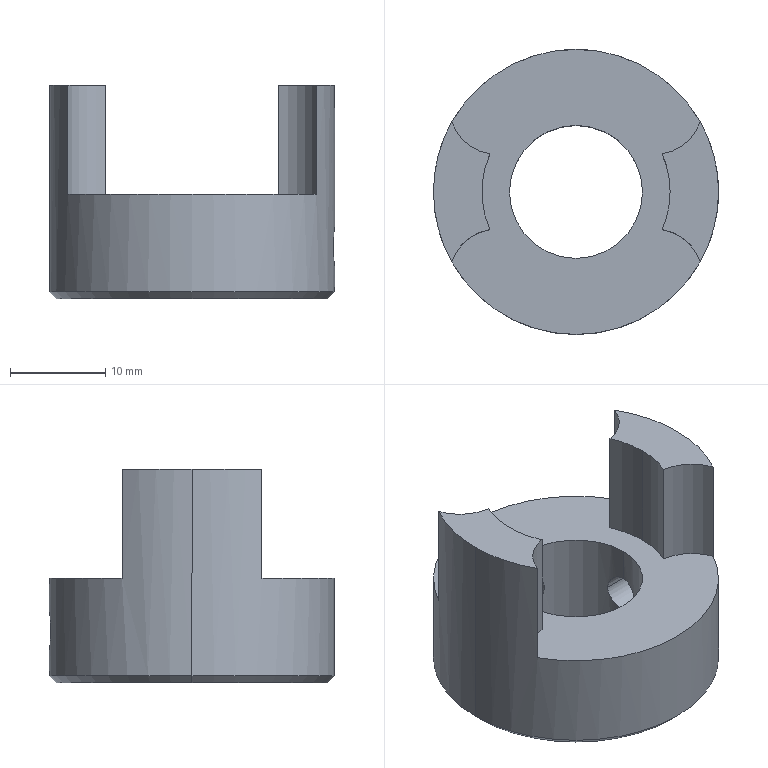Part | SolidWorks | features BaseBody 1 | 1 solid | 21 faces | box 30 x 30 x 22.5 mm | volume 7120 mm3 | cylinder 15 | plane 4 | cone 2 | commonest cylinder face diameters 4 x4 10 x4 19.8 x3 14 x2 30 x2
STEP:
#1=CARTESIAN_POINT('',(0.,15.,-14.));
#2=VERTEX_POINT('',#1);
#3=CARTESIAN_POINT('',(0.,15.,-10.));
#4=VERTEX_POINT('',#3);
#5=CARTESIAN_POINT('',(0.,15.,-14.));
#6=CARTESIAN_POINT('',(0.1323,15.,-14.));
#7=CARTESIAN_POINT('',(0.2623,14.998,-13.987));
#8=CARTESIAN_POINT('',(0.5181,14.992,-13.936));
#9=CARTESIAN_POINT('',(0.6452,14.987,-13.898));
#10=CARTESIAN_POINT('',(0.8873,14.974,-13.797));
#11=CARTESIAN_POINT('',(1.002,14.967,-13.736));
#12=CARTESIAN_POINT('',(1.219,14.951,-13.591));
#13=CARTESIAN_POINT('',(1.322,14.942,-13.506));
#14=CARTESIAN_POINT('',(1.599,14.916,-13.23));
#15=CARTESIAN_POINT('',(1.747,14.898,-13.007));
#16=CARTESIAN_POINT('',(1.947,14.873,-12.526));
#17=CARTESIAN_POINT('',(2.,14.866,-12.263));
#18=CARTESIAN_POINT('',(2.,14.866,-11.871));
#19=CARTESIAN_POINT('',(1.987,14.868,-11.738));
#20=CARTESIAN_POINT('',(1.936,14.875,-11.482));
#21=CARTESIAN_POINT('',(1.898,14.879,-11.357));
#22=CARTESIAN_POINT('',(1.798,14.892,-11.115));
#23=CARTESIAN_POINT('',(1.736,14.899,-10.998));
#24=CARTESIAN_POINT('',(1.591,14.916,-10.781));
#25=CARTESIAN_POINT('',(1.508,14.924,-10.68));
#26=CARTESIAN_POINT('',(1.322,14.942,-10.493));
#27=CARTESIAN_POINT('',(1.221,14.951,-10.411));
#28=CARTESIAN_POINT('',(1.005,14.967,-10.266));
#29=CARTESIAN_POINT('',(0.8878,14.974,-10.203));
#30=CARTESIAN_POINT('',(0.6458,14.987,-10.103));
#31=CARTESIAN_POINT('',(0.5212,14.991,-10.065));
#32=CARTESIAN_POINT('',(0.2647,14.998,-10.013));
#33=CARTESIAN_POINT('',(0.1323,15.,-10.));
#34=CARTESIAN_POINT('',(0.,15.,-10.));
#35=B_SPLINE_CURVE_WITH_KNOTS('',3,(#5,#6,#7,#8,#9,#10,#11,#12,#13,#14,#15,#16,#17,#18,#19,#20,#21,#22,#23,#24,#25,#26,#27,#28,#29,#30,#31,#32,#33,#34),.UNSPECIFIED.,.F.,.F.,(4,2,2,2,2,2,2,2,2,2,2,2,2,2,4),(0.006258,0.00665,0.007041,0.007432,0.007823,0.008605,0.009388,0.009779,0.01017,0.01056,0.01095,0.01134,0.01173,0.01213,0.01252),.UNSPECIFIED.);
#36=EDGE_CURVE('',#2,#4,#35,.T.);
#37=ORIENTED_EDGE('',*,*,#36,.T.);
#38=CARTESIAN_POINT('',(0.,15.,-10.));
#39=CARTESIAN_POINT('',(-0.1323,15.,-10.));
#40=CARTESIAN_POINT('',(-0.2623,14.998,-10.013));
#41=CARTESIAN_POINT('',(-0.5181,14.992,-10.064));
#42=CARTESIAN_POINT('',(-0.6452,14.987,-10.102));
#43=CARTESIAN_POINT('',(-0.8873,14.974,-10.203));
#44=CARTESIAN_POINT('',(-1.002,14.967,-10.264));
#45=CARTESIAN_POINT('',(-1.219,14.951,-10.409));
#46=CARTESIAN_POINT('',(-1.322,14.942,-10.494));
#47=CARTESIAN_POINT('',(-1.599,14.916,-10.77));
#48=CARTESIAN_POINT('',(-1.747,14.898,-10.993));
#49=CARTESIAN_POINT('',(-1.947,14.873,-11.474));
#50=CARTESIAN_POINT('',(-2.,14.866,-11.737));
#51=CARTESIAN_POINT('',(-2.,14.866,-12.129));
#52=CARTESIAN_POINT('',(-1.987,14.868,-12.262));
#53=CARTESIAN_POINT('',(-1.936,14.875,-12.518));
#54=CARTESIAN_POINT('',(-1.898,14.879,-12.643));
#55=CARTESIAN_POINT('',(-1.798,14.892,-12.885));
#56=CARTESIAN_POINT('',(-1.736,14.899,-13.002));
#57=CARTESIAN_POINT('',(-1.591,14.916,-13.219));
#58=CARTESIAN_POINT('',(-1.508,14.924,-13.32));
#59=CARTESIAN_POINT('',(-1.322,14.942,-13.507));
#60=CARTESIAN_POINT('',(-1.221,14.951,-13.589));
#61=CARTESIAN_POINT('',(-1.005,14.967,-13.734));
#62=CARTESIAN_POINT('',(-0.8878,14.974,-13.797));
#63=CARTESIAN_POINT('',(-0.6458,14.987,-13.897));
#64=CARTESIAN_POINT('',(-0.5212,14.991,-13.935));
#65=CARTESIAN_POINT('',(-0.2647,14.998,-13.987));
#66=CARTESIAN_POINT('',(-0.1323,15.,-14.));
#67=CARTESIAN_POINT('',(0.,15.,-14.));
#68=B_SPLINE_CURVE_WITH_KNOTS('',3,(#38,#39,#40,#41,#42,#43,#44,#45,#46,#47,#48,#49,#50,#51,#52,#53,#54,#55,#56,#57,#58,#59,#60,#61,#62,#63,#64,#65,#66,#67),.UNSPECIFIED.,.F.,.F.,(4,2,2,2,2,2,2,2,2,2,2,2,2,2,4),(0.,0.0003912,0.0007823,0.001173,0.001565,0.002347,0.003129,0.00352,0.003912,0.004303,0.004694,0.005085,0.005476,0.005867,0.006258),.UNSPECIFIED.);
#69=EDGE_CURVE('',#4,#2,#68,.T.);
#70=ORIENTED_EDGE('',*,*,#69,.T.);
#71=EDGE_LOOP('',(#37,#70));
#72=FACE_BOUND('',#71,.T.);
#73=CARTESIAN_POINT('',(13.067,7.366,5.));
#74=VERTEX_POINT('',#73);
#75=CARTESIAN_POINT('',(15.,0.,5.));
#76=VERTEX_POINT('',#75);
#77=CARTESIAN_POINT('',(0.,0.,5.));
#78=DIRECTION('',(0.,0.,-1.));
#79=DIRECTION('',(-1.,0.,0.));
#80=AXIS2_PLACEMENT_3D('',#77,#78,#79);
#81=CIRCLE('',#80,15.);
#82=EDGE_CURVE('',#74,#76,#81,.T.);
#83=ORIENTED_EDGE('',*,*,#82,.T.);
#84=CARTESIAN_POINT('',(15.,0.,-10.));
#85=VERTEX_POINT('',#84);
#86=CARTESIAN_POINT('',(15.,0.,-11.625));
#87=DIRECTION('',(0.,0.,-1.));
#88=VECTOR('',#87,1000.);
#89=LINE('',#86,#88);
#90=EDGE_CURVE('',#76,#85,#89,.T.);
#91=ORIENTED_EDGE('',*,*,#90,.T.);
#92=CARTESIAN_POINT('',(14.866,2.,-12.));
#93=VERTEX_POINT('',#92);
#94=CARTESIAN_POINT('',(15.,0.,-10.));
#95=CARTESIAN_POINT('',(15.,0.1322,-10.));
#96=CARTESIAN_POINT('',(14.998,0.2622,-10.013));
#97=CARTESIAN_POINT('',(14.992,0.5179,-10.064));
#98=CARTESIAN_POINT('',(14.987,0.6449,-10.102));
#99=CARTESIAN_POINT('',(14.974,0.8869,-10.203));
#100=CARTESIAN_POINT('',(14.967,1.002,-10.264));
#101=CARTESIAN_POINT('',(14.951,1.219,-10.409));
#102=CARTESIAN_POINT('',(14.942,1.322,-10.493));
#103=CARTESIAN_POINT('',(14.916,1.598,-10.769));
#104=CARTESIAN_POINT('',(14.898,1.747,-10.992));
#105=CARTESIAN_POINT('',(14.873,1.947,-11.473));
#106=CARTESIAN_POINT('',(14.866,2.,-11.736));
#107=CARTESIAN_POINT('',(14.866,2.,-12.));
#108=B_SPLINE_CURVE_WITH_KNOTS('',3,(#94,#95,#96,#97,#98,#99,#100,#101,#102,#103,#104,#105,#106,#107),.UNSPECIFIED.,.F.,.F.,(4,2,2,2,2,2,4),(0.006256,0.006647,0.007038,0.007429,0.00782,0.008602,0.009384),.UNSPECIFIED.);
#109=EDGE_CURVE('',#85,#93,#108,.T.);
#110=ORIENTED_EDGE('',*,*,#109,.T.);
#111=CARTESIAN_POINT('',(15.,0.,-14.));
#112=VERTEX_POINT('',#111);
#113=CARTESIAN_POINT('',(14.866,2.,-12.));
#114=CARTESIAN_POINT('',(14.866,2.,-12.132));
#115=CARTESIAN_POINT('',(14.868,1.987,-12.262));
#116=CARTESIAN_POINT('',(14.875,1.936,-12.518));
#117=CARTESIAN_POINT('',(14.88,1.898,-12.645));
#118=CARTESIAN_POINT('',(14.892,1.797,-12.887));
#119=CARTESIAN_POINT('',(14.899,1.736,-13.002));
#120=CARTESIAN_POINT('',(14.916,1.591,-13.219));
#121=CARTESIAN_POINT('',(14.924,1.507,-13.322));
#122=CARTESIAN_POINT('',(14.951,1.231,-13.598));
#123=CARTESIAN_POINT('',(14.968,1.008,-13.747));
#124=CARTESIAN_POINT('',(14.993,0.5271,-13.947));
#125=CARTESIAN_POINT('',(15.,0.2644,-14.));
#126=CARTESIAN_POINT('',(15.,0.,-14.));
#127=B_SPLINE_CURVE_WITH_KNOTS('',3,(#113,#114,#115,#116,#117,#118,#119,#120,#121,#122,#123,#124,#125,#126),.UNSPECIFIED.,.F.,.F.,(4,2,2,2,2,2,4),(-0.003128,-0.002737,-0.002346,-0.001955,-0.001564,-0.0007819,0.),.UNSPECIFIED.);
#128=EDGE_CURVE('',#93,#112,#127,.T.);
#129=ORIENTED_EDGE('',*,*,#128,.T.);
#130=CARTESIAN_POINT('',(15.,0.,-16.75));
#131=VERTEX_POINT('',#130);
#132=CARTESIAN_POINT('',(15.,0.,-11.625));
#133=DIRECTION('',(0.,0.,-1.));
#134=VECTOR('',#133,1000.);
#135=LINE('',#132,#134);
#136=EDGE_CURVE('',#112,#131,#135,.T.);
#137=ORIENTED_EDGE('',*,*,#136,.T.);
#138=CARTESIAN_POINT('',(-15.,0.,-16.75));
#139=VERTEX_POINT('',#138);
#140=CARTESIAN_POINT('',(0.,0.,-16.75));
#141=DIRECTION('',(0.,0.,1.));
#142=DIRECTION('',(-1.,0.,0.));
#143=AXIS2_PLACEMENT_3D('',#140,#141,#142);
#144=CIRCLE('',#143,15.);
#145=EDGE_CURVE('',#131,#139,#144,.T.);
#146=ORIENTED_EDGE('',*,*,#145,.T.);
#147=CARTESIAN_POINT('',(-15.,0.,5.));
#148=VERTEX_POINT('',#147);
#149=CARTESIAN_POINT('',(-15.,0.,-11.625));
#150=DIRECTION('',(0.,0.,-1.));
#151=VECTOR('',#150,1000.);
#152=LINE('',#149,#151);
#153=EDGE_CURVE('',#148,#139,#152,.T.);
#154=ORIENTED_EDGE('',*,*,#153,.F.);
#155=CARTESIAN_POINT('',(-13.067,7.366,5.));
#156=VERTEX_POINT('',#155);
#157=CARTESIAN_POINT('',(0.,0.,5.));
#158=DIRECTION('',(0.,0.,-1.));
#159=DIRECTION('',(-1.,0.,0.));
#160=AXIS2_PLACEMENT_3D('',#157,#158,#159);
#161=CIRCLE('',#160,15.);
#162=EDGE_CURVE('',#148,#156,#161,.T.);
#163=ORIENTED_EDGE('',*,*,#162,.T.);
#164=CARTESIAN_POINT('',(-13.067,7.366,-6.5));
#165=VERTEX_POINT('',#164);
#166=CARTESIAN_POINT('',(-13.067,7.366,-11.625));
#167=DIRECTION('',(0.,0.,-1.));
#168=VECTOR('',#167,1000.);
#169=LINE('',#166,#168);
#170=EDGE_CURVE('',#156,#165,#169,.T.);
#171=ORIENTED_EDGE('',*,*,#170,.T.);
#172=CARTESIAN_POINT('',(13.067,7.366,-6.5));
#173=VERTEX_POINT('',#172);
#174=CARTESIAN_POINT('',(0.,0.,-6.5));
#175=DIRECTION('',(0.,0.,-1.));
#176=DIRECTION('',(-1.,0.,0.));
#177=AXIS2_PLACEMENT_3D('',#174,#175,#176);
#178=CIRCLE('',#177,15.);
#179=EDGE_CURVE('',#165,#173,#178,.T.);
#180=ORIENTED_EDGE('',*,*,#179,.T.);
#181=CARTESIAN_POINT('',(13.067,7.366,-11.625));
#182=DIRECTION('',(0.,0.,1.));
#183=VECTOR('',#182,1000.);
#184=LINE('',#181,#183);
#185=EDGE_CURVE('',#173,#74,#184,.T.);
#186=ORIENTED_EDGE('',*,*,#185,.T.);
#187=EDGE_LOOP('',(#83,#91,#110,#129,#137,#146,#154,#163,#171,#180,#186));
#188=FACE_OUTER_BOUND('',#187,.T.);
#189=CARTESIAN_POINT('',(0.,0.,-11.625));
#190=DIRECTION('',(0.,0.,-1.));
#191=DIRECTION('',(-1.,0.,0.));
#192=AXIS2_PLACEMENT_3D('',#189,#190,#191);
#193=CYLINDRICAL_SURFACE('',#192,15.);
#194=ADVANCED_FACE('',(#72,#188),#193,.T.);
#195=ORIENTED_EDGE('',*,*,#128,.F.);
#196=CARTESIAN_POINT('',(6.708,2.,-12.));
#197=VERTEX_POINT('',#196);
#198=CARTESIAN_POINT('',(7.5,2.,-12.));
#199=DIRECTION('',(-1.,0.,0.));
#200=VECTOR('',#199,1000.);
#201=LINE('',#198,#200);
#202=EDGE_CURVE('',#93,#197,#201,.T.);
#203=ORIENTED_EDGE('',*,*,#202,.T.);
#204=CARTESIAN_POINT('',(7.,0.,-14.));
#205=VERTEX_POINT('',#204);
#206=CARTESIAN_POINT('',(7.,0.,-14.));
#207=CARTESIAN_POINT('',(7.,0.1328,-14.));
#208=CARTESIAN_POINT('',(6.996,0.2633,-13.987));
#209=CARTESIAN_POINT('',(6.982,0.5197,-13.936));
#210=CARTESIAN_POINT('',(6.971,0.647,-13.897));
#211=CARTESIAN_POINT('',(6.944,0.8888,-13.796));
#212=CARTESIAN_POINT('',(6.929,1.003,-13.735));
#213=CARTESIAN_POINT('',(6.894,1.22,-13.59));
#214=CARTESIAN_POINT('',(6.875,1.322,-13.506));
#215=CARTESIAN_POINT('',(6.818,1.597,-13.231));
#216=CARTESIAN_POINT('',(6.78,1.746,-13.009));
#217=CARTESIAN_POINT('',(6.725,1.946,-12.529));
#218=CARTESIAN_POINT('',(6.708,2.,-12.266));
#219=CARTESIAN_POINT('',(6.708,2.,-12.));
#220=B_SPLINE_CURVE_WITH_KNOTS('',3,(#206,#207,#208,#209,#210,#211,#212,#213,#214,#215,#216,#217,#218,#219),.UNSPECIFIED.,.F.,.F.,(4,2,2,2,2,2,4),(0.006282,0.006674,0.007067,0.00746,0.007852,0.008637,0.009423),.UNSPECIFIED.);
#221=EDGE_CURVE('',#205,#197,#220,.T.);
#222=ORIENTED_EDGE('',*,*,#221,.F.);
#223=CARTESIAN_POINT('',(6.708,-2.,-12.));
#224=VERTEX_POINT('',#223);
#225=CARTESIAN_POINT('',(6.708,-2.,-12.));
#226=CARTESIAN_POINT('',(6.708,-2.,-12.133));
#227=CARTESIAN_POINT('',(6.712,-1.987,-12.263));
#228=CARTESIAN_POINT('',(6.727,-1.936,-12.52));
#229=CARTESIAN_POINT('',(6.738,-1.897,-12.647));
#230=CARTESIAN_POINT('',(6.766,-1.796,-12.889));
#231=CARTESIAN_POINT('',(6.782,-1.735,-13.003));
#232=CARTESIAN_POINT('',(6.817,-1.59,-13.22));
#233=CARTESIAN_POINT('',(6.837,-1.506,-13.322));
#234=CARTESIAN_POINT('',(6.893,-1.231,-13.597));
#235=CARTESIAN_POINT('',(6.931,-1.01,-13.746));
#236=CARTESIAN_POINT('',(6.984,-0.5292,-13.946));
#237=CARTESIAN_POINT('',(7.,-0.2656,-14.));
#238=CARTESIAN_POINT('',(7.,0.,-14.));
#239=B_SPLINE_CURVE_WITH_KNOTS('',3,(#225,#226,#227,#228,#229,#230,#231,#232,#233,#234,#235,#236,#237,#238),.UNSPECIFIED.,.F.,.F.,(4,2,2,2,2,2,4),(0.003141,0.003533,0.003926,0.004319,0.004711,0.005497,0.006282),.UNSPECIFIED.);
#240=EDGE_CURVE('',#224,#205,#239,.T.);
#241=ORIENTED_EDGE('',*,*,#240,.F.);
#242=CARTESIAN_POINT('',(14.866,-2.,-12.));
#243=VERTEX_POINT('',#242);
#244=CARTESIAN_POINT('',(7.5,-2.,-12.));
#245=DIRECTION('',(-1.,0.,0.));
#246=VECTOR('',#245,1000.);
#247=LINE('',#244,#246);
#248=EDGE_CURVE('',#243,#224,#247,.T.);
#249=ORIENTED_EDGE('',*,*,#248,.F.);
#250=CARTESIAN_POINT('',(15.,0.,-14.));
#251=CARTESIAN_POINT('',(15.,-0.1322,-14.));
#252=CARTESIAN_POINT('',(14.998,-0.2622,-13.987));
#253=CARTESIAN_POINT('',(14.992,-0.5179,-13.936));
#254=CARTESIAN_POINT('',(14.987,-0.6449,-13.898));
#255=CARTESIAN_POINT('',(14.974,-0.8869,-13.797));
#256=CARTESIAN_POINT('',(14.967,-1.002,-13.736));
#257=CARTESIAN_POINT('',(14.951,-1.219,-13.591));
#258=CARTESIAN_POINT('',(14.942,-1.322,-13.507));
#259=CARTESIAN_POINT('',(14.916,-1.598,-13.231));
#260=CARTESIAN_POINT('',(14.898,-1.747,-13.008));
#261=CARTESIAN_POINT('',(14.873,-1.947,-12.527));
#262=CARTESIAN_POINT('',(14.866,-2.,-12.264));
#263=CARTESIAN_POINT('',(14.866,-2.,-12.));
#264=B_SPLINE_CURVE_WITH_KNOTS('',3,(#250,#251,#252,#253,#254,#255,#256,#257,#258,#259,#260,#261,#262,#263),.UNSPECIFIED.,.F.,.F.,(4,2,2,2,2,2,4),(0.,0.000391,0.0007819,0.001173,0.001564,0.002346,0.003128),.UNSPECIFIED.);
#265=EDGE_CURVE('',#112,#243,#264,.T.);
#266=ORIENTED_EDGE('',*,*,#265,.F.);
#267=EDGE_LOOP('',(#195,#203,#222,#241,#249,#266));
#268=FACE_OUTER_BOUND('',#267,.T.);
#269=CARTESIAN_POINT('',(7.5,0.,-12.));
#270=DIRECTION('',(-1.,0.,0.));
#271=DIRECTION('',(0.,-1.,0.));
#272=AXIS2_PLACEMENT_3D('',#269,#270,#271);
#273=CYLINDRICAL_SURFACE('',#272,2.);
#274=ADVANCED_FACE('',(#268),#273,.F.);
#275=CARTESIAN_POINT('',(14.25,0.,-17.5));
#276=VERTEX_POINT('',#275);
#277=CARTESIAN_POINT('',(-14.25,0.,-17.5));
#278=VERTEX_POINT('',#277);
#279=CARTESIAN_POINT('',(0.,0.,-17.5));
#280=DIRECTION('',(0.,0.,1.));
#281=DIRECTION('',(1.,0.,0.));
#282=AXIS2_PLACEMENT_3D('',#279,#280,#281);
#283=CIRCLE('',#282,14.25);
#284=EDGE_CURVE('',#276,#278,#283,.T.);
#285=ORIENTED_EDGE('',*,*,#284,.T.);
#286=CARTESIAN_POINT('',(-15.,0.,-16.75));
#287=DIRECTION('',(-0.7071,0.,0.7071));
#288=VECTOR('',#287,1000.);
#289=LINE('',#286,#288);
#290=EDGE_CURVE('',#278,#139,#289,.T.);
#291=ORIENTED_EDGE('',*,*,#290,.T.);
#292=ORIENTED_EDGE('',*,*,#145,.F.);
#293=CARTESIAN_POINT('',(15.,0.,-16.75));
#294=DIRECTION('',(0.7071,0.,0.7071));
#295=VECTOR('',#294,1000.);
#296=LINE('',#293,#295);
#297=EDGE_CURVE('',#276,#131,#296,.T.);
#298=ORIENTED_EDGE('',*,*,#297,.F.);
#299=EDGE_LOOP('',(#285,#291,#292,#298));
#300=FACE_OUTER_BOUND('',#299,.T.);
#301=CARTESIAN_POINT('',(0.,0.,-16.75));
#302=DIRECTION('',(0.,0.,1.));
#303=DIRECTION('',(1.,0.,0.));
#304=AXIS2_PLACEMENT_3D('',#301,#302,#303);
#305=CONICAL_SURFACE('',#304,15.,0.7854);
#306=ADVANCED_FACE('',(#300),#305,.T.);
#307=CARTESIAN_POINT('',(7.,0.,-6.5));
#308=VERTEX_POINT('',#307);
#309=CARTESIAN_POINT('',(-7.,0.,-6.5));
#310=VERTEX_POINT('',#309);
#311=CARTESIAN_POINT('',(0.,0.,-6.5));
#312=DIRECTION('',(0.,0.,-1.));
#313=DIRECTION('',(-1.,0.,0.));
#314=AXIS2_PLACEMENT_3D('',#311,#312,#313);
#315=CIRCLE('',#314,7.);
#316=EDGE_CURVE('',#308,#310,#315,.T.);
#317=ORIENTED_EDGE('',*,*,#316,.F.);
#318=CARTESIAN_POINT('',(7.,0.,-10.));
#319=VERTEX_POINT('',#318);
#320=CARTESIAN_POINT('',(7.,0.,5.));
#321=DIRECTION('',(0.,0.,-1.));
#322=VECTOR('',#321,1000.);
#323=LINE('',#320,#322);
#324=EDGE_CURVE('',#308,#319,#323,.T.);
#325=ORIENTED_EDGE('',*,*,#324,.T.);
#326=CARTESIAN_POINT('',(7.,0.,-10.));
#327=CARTESIAN_POINT('',(7.,-0.1328,-10.));
#328=CARTESIAN_POINT('',(6.996,-0.2633,-10.013));
#329=CARTESIAN_POINT('',(6.982,-0.5197,-10.064));
#330=CARTESIAN_POINT('',(6.971,-0.647,-10.103));
#331=CARTESIAN_POINT('',(6.944,-0.8888,-10.204));
#332=CARTESIAN_POINT('',(6.929,-1.003,-10.265));
#333=CARTESIAN_POINT('',(6.894,-1.22,-10.41));
#334=CARTESIAN_POINT('',(6.875,-1.322,-10.494));
#335=CARTESIAN_POINT('',(6.818,-1.597,-10.769));
#336=CARTESIAN_POINT('',(6.78,-1.746,-10.991));
#337=CARTESIAN_POINT('',(6.725,-1.946,-11.471));
#338=CARTESIAN_POINT('',(6.708,-2.,-11.734));
#339=CARTESIAN_POINT('',(6.708,-2.,-12.));
#340=B_SPLINE_CURVE_WITH_KNOTS('',3,(#326,#327,#328,#329,#330,#331,#332,#333,#334,#335,#336,#337,#338,#339),.UNSPECIFIED.,.F.,.F.,(4,2,2,2,2,2,4),(0.,0.0003926,0.0007852,0.001178,0.00157,0.002356,0.003141),.UNSPECIFIED.);
#341=EDGE_CURVE('',#319,#224,#340,.T.);
#342=ORIENTED_EDGE('',*,*,#341,.T.);
#343=ORIENTED_EDGE('',*,*,#240,.T.);
#344=CARTESIAN_POINT('',(7.,0.,-17.5));
#345=VERTEX_POINT('',#344);
#346=CARTESIAN_POINT('',(7.,0.,5.));
#347=DIRECTION('',(0.,0.,-1.));
#348=VECTOR('',#347,1000.);
#349=LINE('',#346,#348);
#350=EDGE_CURVE('',#205,#345,#349,.T.);
#351=ORIENTED_EDGE('',*,*,#350,.T.);
#352=CARTESIAN_POINT('',(-7.,0.,-17.5));
#353=VERTEX_POINT('',#352);
#354=CARTESIAN_POINT('',(0.,0.,-17.5));
#355=DIRECTION('',(0.,0.,1.));
#356=DIRECTION('',(-1.,0.,0.));
#357=AXIS2_PLACEMENT_3D('',#354,#355,#356);
#358=CIRCLE('',#357,7.);
#359=EDGE_CURVE('',#353,#345,#358,.T.);
#360=ORIENTED_EDGE('',*,*,#359,.F.);
#361=CARTESIAN_POINT('',(-7.,0.,5.));
#362=DIRECTION('',(0.,0.,-1.));
#363=VECTOR('',#362,1000.);
#364=LINE('',#361,#363);
#365=EDGE_CURVE('',#310,#353,#364,.T.);
#366=ORIENTED_EDGE('',*,*,#365,.F.);
#367=EDGE_LOOP('',(#317,#325,#342,#343,#351,#360,#366));
#368=FACE_OUTER_BOUND('',#367,.T.);
#369=CARTESIAN_POINT('',(0.,0.,5.));
#370=DIRECTION('',(0.,0.,-1.));
#371=DIRECTION('',(-1.,0.,0.));
#372=AXIS2_PLACEMENT_3D('',#369,#370,#371);
#373=CYLINDRICAL_SURFACE('',#372,7.);
#374=ADVANCED_FACE('',(#368),#373,.F.);
#375=ORIENTED_EDGE('',*,*,#69,.F.);
#376=CARTESIAN_POINT('',(0.,7.,-10.));
#377=VERTEX_POINT('',#376);
#378=CARTESIAN_POINT('',(0.,7.5,-10.));
#379=DIRECTION('',(0.,-1.,0.));
#380=VECTOR('',#379,1000.);
#381=LINE('',#378,#380);
#382=EDGE_CURVE('',#4,#377,#381,.T.);
#383=ORIENTED_EDGE('',*,*,#382,.T.);
#384=CARTESIAN_POINT('',(0.,7.,-14.));
#385=VERTEX_POINT('',#384);
#386=CARTESIAN_POINT('',(0.,7.,-10.));
#387=CARTESIAN_POINT('',(-0.1328,7.,-10.));
#388=CARTESIAN_POINT('',(-0.2633,6.996,-10.013));
#389=CARTESIAN_POINT('',(-0.5199,6.982,-10.064));
#390=CARTESIAN_POINT('',(-0.6472,6.971,-10.103));
#391=CARTESIAN_POINT('',(-0.8891,6.944,-10.204));
#392=CARTESIAN_POINT('',(-1.004,6.929,-10.265));
#393=CARTESIAN_POINT('',(-1.221,6.894,-10.41));
#394=CARTESIAN_POINT('',(-1.323,6.875,-10.494));
#395=CARTESIAN_POINT('',(-1.598,6.818,-10.769));
#396=CARTESIAN_POINT('',(-1.746,6.779,-10.991));
#397=CARTESIAN_POINT('',(-1.896,6.738,-11.352));
#398=CARTESIAN_POINT('',(-1.935,6.727,-11.478));
#399=CARTESIAN_POINT('',(-1.987,6.712,-11.737));
#400=CARTESIAN_POINT('',(-2.,6.708,-11.867));
#401=CARTESIAN_POINT('',(-2.,6.708,-12.129));
#402=CARTESIAN_POINT('',(-1.987,6.712,-12.263));
#403=CARTESIAN_POINT('',(-1.936,6.727,-12.52));
#404=CARTESIAN_POINT('',(-1.898,6.738,-12.645));
#405=CARTESIAN_POINT('',(-1.747,6.779,-13.009));
#406=CARTESIAN_POINT('',(-1.6,6.817,-13.229));
#407=CARTESIAN_POINT('',(-1.323,6.875,-13.506));
#408=CARTESIAN_POINT('',(-1.222,6.893,-13.588));
#409=CARTESIAN_POINT('',(-1.006,6.928,-13.733));
#410=CARTESIAN_POINT('',(-0.8894,6.944,-13.796));
#411=CARTESIAN_POINT('',(-0.6484,6.971,-13.896));
#412=CARTESIAN_POINT('',(-0.5237,6.982,-13.935));
#413=CARTESIAN_POINT('',(-0.2658,6.996,-13.987));
#414=CARTESIAN_POINT('',(-0.1328,7.,-14.));
#415=CARTESIAN_POINT('',(0.,7.,-14.));
#416=B_SPLINE_CURVE_WITH_KNOTS('',3,(#386,#387,#388,#389,#390,#391,#392,#393,#394,#395,#396,#397,#398,#399,#400,#401,#402,#403,#404,#405,#406,#407,#408,#409,#410,#411,#412,#413,#414,#415),.UNSPECIFIED.,.F.,.F.,(4,2,2,2,2,2,2,2,2,2,2,2,2,2,4),(0.006284,0.006676,0.007069,0.007462,0.007855,0.00864,0.009033,0.009425,0.009818,0.01021,0.011,0.01139,0.01178,0.01217,0.01257),.UNSPECIFIED.);
#417=EDGE_CURVE('',#377,#385,#416,.T.);
#418=ORIENTED_EDGE('',*,*,#417,.T.);
#419=CARTESIAN_POINT('',(0.,7.5,-14.));
#420=DIRECTION('',(0.,-1.,0.));
#421=VECTOR('',#420,1000.);
#422=LINE('',#419,#421);
#423=EDGE_CURVE('',#2,#385,#422,.T.);
#424=ORIENTED_EDGE('',*,*,#423,.F.);
#425=EDGE_LOOP('',(#375,#383,#418,#424));
#426=FACE_OUTER_BOUND('',#425,.T.);
#427=CARTESIAN_POINT('',(0.,7.5,-12.));
#428=DIRECTION('',(0.,-1.,0.));
#429=DIRECTION('',(0.,0.,-1.));
#430=AXIS2_PLACEMENT_3D('',#427,#428,#429);
#431=CYLINDRICAL_SURFACE('',#430,2.);
#432=ADVANCED_FACE('',(#426),#431,.F.);
#433=CARTESIAN_POINT('',(9.9,0.,-6.5));
#434=VERTEX_POINT('',#433);
#435=CARTESIAN_POINT('',(9.056,4.,-6.5));
#436=VERTEX_POINT('',#435);
#437=CARTESIAN_POINT('',(0.,0.,-6.5));
#438=DIRECTION('',(0.,0.,1.));
#439=DIRECTION('',(1.,0.,0.));
#440=AXIS2_PLACEMENT_3D('',#437,#438,#439);
#441=CIRCLE('',#440,9.9);
#442=EDGE_CURVE('',#434,#436,#441,.T.);
#443=ORIENTED_EDGE('',*,*,#442,.F.);
#444=CARTESIAN_POINT('',(9.9,0.,5.));
#445=VERTEX_POINT('',#444);
#446=CARTESIAN_POINT('',(9.9,0.,-6.5));
#447=DIRECTION('',(0.,0.,1.));
#448=VECTOR('',#447,1000.);
#449=LINE('',#446,#448);
#450=EDGE_CURVE('',#434,#445,#449,.T.);
#451=ORIENTED_EDGE('',*,*,#450,.T.);
#452=CARTESIAN_POINT('',(9.056,4.,5.));
#453=VERTEX_POINT('',#452);
#454=CARTESIAN_POINT('',(0.,0.,5.));
#455=DIRECTION('',(0.,0.,-1.));
#456=DIRECTION('',(1.,0.,0.));
#457=AXIS2_PLACEMENT_3D('',#454,#455,#456);
#458=CIRCLE('',#457,9.9);
#459=EDGE_CURVE('',#453,#445,#458,.T.);
#460=ORIENTED_EDGE('',*,*,#459,.F.);
#461=CARTESIAN_POINT('',(9.056,4.,-6.5));
#462=DIRECTION('',(0.,0.,-1.));
#463=VECTOR('',#462,1000.);
#464=LINE('',#461,#463);
#465=EDGE_CURVE('',#453,#436,#464,.T.);
#466=ORIENTED_EDGE('',*,*,#465,.T.);
#467=EDGE_LOOP('',(#443,#451,#460,#466));
#468=FACE_OUTER_BOUND('',#467,.T.);
#469=CARTESIAN_POINT('',(0.,0.,-6.5));
#470=DIRECTION('',(0.,0.,1.));
#471=DIRECTION('',(1.,0.,0.));
#472=AXIS2_PLACEMENT_3D('',#469,#470,#471);
#473=CYLINDRICAL_SURFACE('',#472,9.9);
#474=ADVANCED_FACE('',(#468),#473,.F.);
#475=ORIENTED_EDGE('',*,*,#90,.F.);
#476=CARTESIAN_POINT('',(13.067,-7.366,5.));
#477=VERTEX_POINT('',#476);
#478=CARTESIAN_POINT('',(0.,0.,5.));
#479=DIRECTION('',(0.,0.,-1.));
#480=DIRECTION('',(-1.,0.,0.));
#481=AXIS2_PLACEMENT_3D('',#478,#479,#480);
#482=CIRCLE('',#481,15.);
#483=EDGE_CURVE('',#76,#477,#482,.T.);
#484=ORIENTED_EDGE('',*,*,#483,.T.);
#485=CARTESIAN_POINT('',(13.067,-7.366,-6.5));
#486=VERTEX_POINT('',#485);
#487=CARTESIAN_POINT('',(13.067,-7.366,-11.625));
#488=DIRECTION('',(0.,0.,-1.));
#489=VECTOR('',#488,1000.);
#490=LINE('',#487,#489);
#491=EDGE_CURVE('',#477,#486,#490,.T.);
#492=ORIENTED_EDGE('',*,*,#491,.T.);
#493=CARTESIAN_POINT('',(-13.067,-7.366,-6.5));
#494=VERTEX_POINT('',#493);
#495=CARTESIAN_POINT('',(0.,0.,-6.5));
#496=DIRECTION('',(0.,0.,-1.));
#497=DIRECTION('',(-1.,0.,0.));
#498=AXIS2_PLACEMENT_3D('',#495,#496,#497);
#499=CIRCLE('',#498,15.);
#500=EDGE_CURVE('',#486,#494,#499,.T.);
#501=ORIENTED_EDGE('',*,*,#500,.T.);
#502=CARTESIAN_POINT('',(-13.067,-7.366,5.));
#503=VERTEX_POINT('',#502);
#504=CARTESIAN_POINT('',(-13.067,-7.366,-11.625));
#505=DIRECTION('',(0.,0.,1.));
#506=VECTOR('',#505,1000.);
#507=LINE('',#504,#506);
#508=EDGE_CURVE('',#494,#503,#507,.T.);
#509=ORIENTED_EDGE('',*,*,#508,.T.);
#510=CARTESIAN_POINT('',(0.,0.,5.));
#511=DIRECTION('',(0.,0.,-1.));
#512=DIRECTION('',(-1.,0.,0.));
#513=AXIS2_PLACEMENT_3D('',#510,#511,#512);
#514=CIRCLE('',#513,15.);
#515=EDGE_CURVE('',#503,#148,#514,.T.);
#516=ORIENTED_EDGE('',*,*,#515,.T.);
#517=ORIENTED_EDGE('',*,*,#153,.T.);
#518=CARTESIAN_POINT('',(0.,0.,-16.75));
#519=DIRECTION('',(0.,0.,1.));
#520=DIRECTION('',(-1.,0.,0.));
#521=AXIS2_PLACEMENT_3D('',#518,#519,#520);
#522=CIRCLE('',#521,15.);
#523=EDGE_CURVE('',#139,#131,#522,.T.);
#524=ORIENTED_EDGE('',*,*,#523,.T.);
#525=ORIENTED_EDGE('',*,*,#136,.F.);
#526=ORIENTED_EDGE('',*,*,#265,.T.);
#527=CARTESIAN_POINT('',(14.866,-2.,-12.));
#528=CARTESIAN_POINT('',(14.866,-2.,-11.868));
#529=CARTESIAN_POINT('',(14.868,-1.987,-11.738));
#530=CARTESIAN_POINT('',(14.875,-1.936,-11.482));
#531=CARTESIAN_POINT('',(14.88,-1.898,-11.355));
#532=CARTESIAN_POINT('',(14.892,-1.797,-11.113));
#533=CARTESIAN_POINT('',(14.899,-1.736,-10.998));
#534=CARTESIAN_POINT('',(14.916,-1.591,-10.781));
#535=CARTESIAN_POINT('',(14.924,-1.507,-10.678));
#536=CARTESIAN_POINT('',(14.951,-1.231,-10.402));
#537=CARTESIAN_POINT('',(14.968,-1.008,-10.253));
#538=CARTESIAN_POINT('',(14.993,-0.5271,-10.053));
#539=CARTESIAN_POINT('',(15.,-0.2644,-10.));
#540=CARTESIAN_POINT('',(15.,0.,-10.));
#541=B_SPLINE_CURVE_WITH_KNOTS('',3,(#527,#528,#529,#530,#531,#532,#533,#534,#535,#536,#537,#538,#539,#540),.UNSPECIFIED.,.F.,.F.,(4,2,2,2,2,2,4),(0.003128,0.003519,0.00391,0.004301,0.004692,0.005474,0.006256),.UNSPECIFIED.);
#542=EDGE_CURVE('',#243,#85,#541,.T.);
#543=ORIENTED_EDGE('',*,*,#542,.T.);
#544=EDGE_LOOP('',(#475,#484,#492,#501,#509,#516,#517,#524,#525,#526,#543));
#545=FACE_OUTER_BOUND('',#544,.T.);
#546=CARTESIAN_POINT('',(0.,0.,-11.625));
#547=DIRECTION('',(0.,0.,-1.));
#548=DIRECTION('',(-1.,0.,0.));
#549=AXIS2_PLACEMENT_3D('',#546,#547,#548);
#550=CYLINDRICAL_SURFACE('',#549,15.);
#551=ADVANCED_FACE('',(#545),#550,.T.);
#552=ORIENTED_EDGE('',*,*,#202,.F.);
#553=ORIENTED_EDGE('',*,*,#109,.F.);
#554=ORIENTED_EDGE('',*,*,#542,.F.);
#555=ORIENTED_EDGE('',*,*,#248,.T.);
#556=ORIENTED_EDGE('',*,*,#341,.F.);
#557=CARTESIAN_POINT('',(6.708,2.,-12.));
#558=CARTESIAN_POINT('',(6.708,2.,-11.867));
#559=CARTESIAN_POINT('',(6.712,1.987,-11.737));
#560=CARTESIAN_POINT('',(6.727,1.936,-11.48));
#561=CARTESIAN_POINT('',(6.738,1.897,-11.353));
#562=CARTESIAN_POINT('',(6.766,1.796,-11.111));
#563=CARTESIAN_POINT('',(6.782,1.735,-10.997));
#564=CARTESIAN_POINT('',(6.817,1.59,-10.78));
#565=CARTESIAN_POINT('',(6.837,1.506,-10.678));
#566=CARTESIAN_POINT('',(6.893,1.231,-10.403));
#567=CARTESIAN_POINT('',(6.931,1.01,-10.254));
#568=CARTESIAN_POINT('',(6.984,0.5292,-10.054));
#569=CARTESIAN_POINT('',(7.,0.2656,-10.));
#570=CARTESIAN_POINT('',(7.,0.,-10.));
#571=B_SPLINE_CURVE_WITH_KNOTS('',3,(#557,#558,#559,#560,#561,#562,#563,#564,#565,#566,#567,#568,#569,#570),.UNSPECIFIED.,.F.,.F.,(4,2,2,2,2,2,4),(-0.003141,-0.002748,-0.002356,-0.001963,-0.00157,-0.0007852,0.),.UNSPECIFIED.);
#572=EDGE_CURVE('',#197,#319,#571,.T.);
#573=ORIENTED_EDGE('',*,*,#572,.F.);
#574=EDGE_LOOP('',(#552,#553,#554,#555,#556,#573));
#575=FACE_OUTER_BOUND('',#574,.T.);
#576=CARTESIAN_POINT('',(7.5,0.,-12.));
#577=DIRECTION('',(-1.,0.,0.));
#578=DIRECTION('',(0.,-1.,0.));
#579=AXIS2_PLACEMENT_3D('',#576,#577,#578);
#580=CYLINDRICAL_SURFACE('',#579,2.);
#581=ADVANCED_FACE('',(#575),#580,.F.);
#582=ORIENTED_EDGE('',*,*,#290,.F.);
#583=CARTESIAN_POINT('',(0.,0.,-17.5));
#584=DIRECTION('',(0.,0.,1.));
#585=DIRECTION('',(1.,0.,0.));
#586=AXIS2_PLACEMENT_3D('',#583,#584,#585);
#587=CIRCLE('',#586,14.25);
#588=EDGE_CURVE('',#278,#276,#587,.T.);
#589=ORIENTED_EDGE('',*,*,#588,.T.);
#590=ORIENTED_EDGE('',*,*,#297,.T.);
#591=ORIENTED_EDGE('',*,*,#523,.F.);
#592=EDGE_LOOP('',(#582,#589,#590,#591));
#593=FACE_OUTER_BOUND('',#592,.T.);
#594=CARTESIAN_POINT('',(0.,0.,-16.75));
#595=DIRECTION('',(0.,0.,1.));
#596=DIRECTION('',(1.,0.,0.));
#597=AXIS2_PLACEMENT_3D('',#594,#595,#596);
#598=CONICAL_SURFACE('',#597,15.,0.7854);
#599=ADVANCED_FACE('',(#593),#598,.T.);
#600=CARTESIAN_POINT('',(-9.056,4.,5.));
#601=VERTEX_POINT('',#600);
#602=CARTESIAN_POINT('',(-8.323,8.946,5.));
#603=DIRECTION('',(0.,0.,-1.));
#604=DIRECTION('',(1.,0.,0.));
#605=AXIS2_PLACEMENT_3D('',#602,#603,#604);
#606=CIRCLE('',#605,5.);
#607=EDGE_CURVE('',#601,#156,#606,.T.);
#608=ORIENTED_EDGE('',*,*,#607,.T.);
#609=ORIENTED_EDGE('',*,*,#162,.F.);
#610=ORIENTED_EDGE('',*,*,#515,.F.);
#611=CARTESIAN_POINT('',(-9.056,-4.,5.));
#612=VERTEX_POINT('',#611);
#613=CARTESIAN_POINT('',(-8.323,-8.946,5.));
#614=DIRECTION('',(0.,0.,-1.));
#615=DIRECTION('',(1.,0.,0.));
#616=AXIS2_PLACEMENT_3D('',#613,#614,#615);
#617=CIRCLE('',#616,5.);
#618=EDGE_CURVE('',#503,#612,#617,.T.);
#619=ORIENTED_EDGE('',*,*,#618,.T.);
#620=CARTESIAN_POINT('',(0.,0.,5.));
#621=DIRECTION('',(0.,0.,-1.));
#622=DIRECTION('',(1.,0.,0.));
#623=AXIS2_PLACEMENT_3D('',#620,#621,#622);
#624=CIRCLE('',#623,9.9);
#625=EDGE_CURVE('',#612,#601,#624,.T.);
#626=ORIENTED_EDGE('',*,*,#625,.T.);
#627=EDGE_LOOP('',(#608,#609,#610,#619,#626));
#628=FACE_OUTER_BOUND('',#627,.T.);
#629=CARTESIAN_POINT('',(-12.2,0.000000001,5.));
#630=DIRECTION('',(0.,0.,1.));
#631=DIRECTION('',(1.,0.,0.));
#632=AXIS2_PLACEMENT_3D('',#629,#630,#631);
#633=PLANE('',#632);
#634=ADVANCED_FACE('',(#628),#633,.T.);
#635=CARTESIAN_POINT('',(-9.056,-4.,-6.5));
#636=VERTEX_POINT('',#635);
#637=CARTESIAN_POINT('',(-8.323,-8.946,-6.5));
#638=DIRECTION('',(0.,0.,1.));
#639=DIRECTION('',(1.,0.,0.));
#640=AXIS2_PLACEMENT_3D('',#637,#638,#639);
#641=CIRCLE('',#640,5.);
#642=EDGE_CURVE('',#636,#494,#641,.T.);
#643=ORIENTED_EDGE('',*,*,#642,.F.);
#644=CARTESIAN_POINT('',(-9.056,-4.,-6.5));
#645=DIRECTION('',(0.,0.,-1.));
#646=VECTOR('',#645,1000.);
#647=LINE('',#644,#646);
#648=EDGE_CURVE('',#612,#636,#647,.T.);
#649=ORIENTED_EDGE('',*,*,#648,.F.);
#650=ORIENTED_EDGE('',*,*,#618,.F.);
#651=ORIENTED_EDGE('',*,*,#508,.F.);
#652=EDGE_LOOP('',(#643,#649,#650,#651));
#653=FACE_OUTER_BOUND('',#652,.T.);
#654=CARTESIAN_POINT('',(-8.323,-8.946,-6.5));
#655=DIRECTION('',(0.,0.,1.));
#656=DIRECTION('',(1.,0.,0.));
#657=AXIS2_PLACEMENT_3D('',#654,#655,#656);
#658=CYLINDRICAL_SURFACE('',#657,5.);
#659=ADVANCED_FACE('',(#653),#658,.F.);
#660=CARTESIAN_POINT('',(8.323,8.946,-6.5));
#661=DIRECTION('',(0.,0.,1.));
#662=DIRECTION('',(1.,0.,0.));
#663=AXIS2_PLACEMENT_3D('',#660,#661,#662);
#664=CIRCLE('',#663,5.);
#665=EDGE_CURVE('',#436,#173,#664,.T.);
#666=ORIENTED_EDGE('',*,*,#665,.T.);
#667=ORIENTED_EDGE('',*,*,#179,.F.);
#668=CARTESIAN_POINT('',(-9.056,4.,-6.5));
#669=VERTEX_POINT('',#668);
#670=CARTESIAN_POINT('',(-8.323,8.946,-6.5));
#671=DIRECTION('',(0.,0.,1.));
#672=DIRECTION('',(1.,0.,0.));
#673=AXIS2_PLACEMENT_3D('',#670,#671,#672);
#674=CIRCLE('',#673,5.);
#675=EDGE_CURVE('',#165,#669,#674,.T.);
#676=ORIENTED_EDGE('',*,*,#675,.T.);
#677=CARTESIAN_POINT('',(0.,0.,-6.5));
#678=DIRECTION('',(0.,0.,1.));
#679=DIRECTION('',(1.,0.,0.));
#680=AXIS2_PLACEMENT_3D('',#677,#678,#679);
#681=CIRCLE('',#680,9.9);
#682=EDGE_CURVE('',#669,#636,#681,.T.);
#683=ORIENTED_EDGE('',*,*,#682,.T.);
#684=ORIENTED_EDGE('',*,*,#642,.T.);
#685=ORIENTED_EDGE('',*,*,#500,.F.);
#686=CARTESIAN_POINT('',(9.056,-4.,-6.5));
#687=VERTEX_POINT('',#686);
#688=CARTESIAN_POINT('',(8.323,-8.946,-6.5));
#689=DIRECTION('',(0.,0.,1.));
#690=DIRECTION('',(1.,0.,0.));
#691=AXIS2_PLACEMENT_3D('',#688,#689,#690);
#692=CIRCLE('',#691,5.);
#693=EDGE_CURVE('',#486,#687,#692,.T.);
#694=ORIENTED_EDGE('',*,*,#693,.T.);
#695=CARTESIAN_POINT('',(0.,0.,-6.5));
#696=DIRECTION('',(0.,0.,1.));
#697=DIRECTION('',(1.,0.,0.));
#698=AXIS2_PLACEMENT_3D('',#695,#696,#697);
#699=CIRCLE('',#698,9.9);
#700=EDGE_CURVE('',#687,#434,#699,.T.);
#701=ORIENTED_EDGE('',*,*,#700,.T.);
#702=ORIENTED_EDGE('',*,*,#442,.T.);
#703=EDGE_LOOP('',(#666,#667,#676,#683,#684,#685,#694,#701,#702));
#704=FACE_OUTER_BOUND('',#703,.T.);
#705=CARTESIAN_POINT('',(0.,0.,-6.5));
#706=DIRECTION('',(0.,0.,-1.));
#707=DIRECTION('',(-1.,0.,0.));
#708=AXIS2_PLACEMENT_3D('',#705,#706,#707);
#709=CIRCLE('',#708,7.);
#710=EDGE_CURVE('',#310,#308,#709,.T.);
#711=ORIENTED_EDGE('',*,*,#710,.T.);
#712=ORIENTED_EDGE('',*,*,#316,.T.);
#713=EDGE_LOOP('',(#711,#712));
#714=FACE_BOUND('',#713,.T.);
#715=CARTESIAN_POINT('',(0.,10.375,-6.5));
#716=DIRECTION('',(0.,0.,1.));
#717=DIRECTION('',(1.,0.,0.));
#718=AXIS2_PLACEMENT_3D('',#715,#716,#717);
#719=PLANE('',#718);
#720=ADVANCED_FACE('',(#704,#714),#719,.T.);
#721=ORIENTED_EDGE('',*,*,#693,.F.);
#722=ORIENTED_EDGE('',*,*,#491,.F.);
#723=CARTESIAN_POINT('',(9.056,-4.,5.));
#724=VERTEX_POINT('',#723);
#725=CARTESIAN_POINT('',(8.323,-8.946,5.));
#726=DIRECTION('',(0.,0.,-1.));
#727=DIRECTION('',(1.,0.,0.));
#728=AXIS2_PLACEMENT_3D('',#725,#726,#727);
#729=CIRCLE('',#728,5.);
#730=EDGE_CURVE('',#724,#477,#729,.T.);
#731=ORIENTED_EDGE('',*,*,#730,.F.);
#732=CARTESIAN_POINT('',(9.056,-4.,-6.5));
#733=DIRECTION('',(0.,0.,1.));
#734=VECTOR('',#733,1000.);
#735=LINE('',#732,#734);
#736=EDGE_CURVE('',#687,#724,#735,.T.);
#737=ORIENTED_EDGE('',*,*,#736,.F.);
#738=EDGE_LOOP('',(#721,#722,#731,#737));
#739=FACE_OUTER_BOUND('',#738,.T.);
#740=CARTESIAN_POINT('',(8.323,-8.946,-6.5));
#741=DIRECTION('',(0.,0.,1.));
#742=DIRECTION('',(1.,0.,0.));
#743=AXIS2_PLACEMENT_3D('',#740,#741,#742);
#744=CYLINDRICAL_SURFACE('',#743,5.);
#745=ADVANCED_FACE('',(#739),#744,.F.);
#746=ORIENTED_EDGE('',*,*,#730,.T.);
#747=ORIENTED_EDGE('',*,*,#483,.F.);
#748=ORIENTED_EDGE('',*,*,#82,.F.);
#749=CARTESIAN_POINT('',(8.323,8.946,5.));
#750=DIRECTION('',(0.,0.,-1.));
#751=DIRECTION('',(1.,0.,0.));
#752=AXIS2_PLACEMENT_3D('',#749,#750,#751);
#753=CIRCLE('',#752,5.);
#754=EDGE_CURVE('',#74,#453,#753,.T.);
#755=ORIENTED_EDGE('',*,*,#754,.T.);
#756=ORIENTED_EDGE('',*,*,#459,.T.);
#757=CARTESIAN_POINT('',(0.,0.,5.));
#758=DIRECTION('',(0.,0.,-1.));
#759=DIRECTION('',(1.,0.,0.));
#760=AXIS2_PLACEMENT_3D('',#757,#758,#759);
#761=CIRCLE('',#760,9.9);
#762=EDGE_CURVE('',#445,#724,#761,.T.);
#763=ORIENTED_EDGE('',*,*,#762,.T.);
#764=EDGE_LOOP('',(#746,#747,#748,#755,#756,#763));
#765=FACE_OUTER_BOUND('',#764,.T.);
#766=CARTESIAN_POINT('',(12.2,-0.000000001,5.));
#767=DIRECTION('',(0.,0.,1.));
#768=DIRECTION('',(1.,0.,0.));
#769=AXIS2_PLACEMENT_3D('',#766,#767,#768);
#770=PLANE('',#769);
#771=ADVANCED_FACE('',(#765),#770,.T.);
#772=ORIENTED_EDGE('',*,*,#324,.F.);
#773=ORIENTED_EDGE('',*,*,#710,.F.);
#774=ORIENTED_EDGE('',*,*,#365,.T.);
#775=CARTESIAN_POINT('',(0.,0.,-17.5));
#776=DIRECTION('',(0.,0.,1.));
#777=DIRECTION('',(-1.,0.,0.));
#778=AXIS2_PLACEMENT_3D('',#775,#776,#777);
#779=CIRCLE('',#778,7.);
#780=EDGE_CURVE('',#345,#353,#779,.T.);
#781=ORIENTED_EDGE('',*,*,#780,.F.);
#782=ORIENTED_EDGE('',*,*,#350,.F.);
#783=ORIENTED_EDGE('',*,*,#221,.T.);
#784=ORIENTED_EDGE('',*,*,#572,.T.);
#785=EDGE_LOOP('',(#772,#773,#774,#781,#782,#783,#784));
#786=FACE_OUTER_BOUND('',#785,.T.);
#787=CARTESIAN_POINT('',(0.,7.,-14.));
#788=CARTESIAN_POINT('',(0.1328,7.,-14.));
#789=CARTESIAN_POINT('',(0.2633,6.996,-13.987));
#790=CARTESIAN_POINT('',(0.5199,6.982,-13.936));
#791=CARTESIAN_POINT('',(0.6472,6.971,-13.897));
#792=CARTESIAN_POINT('',(0.8891,6.944,-13.796));
#793=CARTESIAN_POINT('',(1.004,6.929,-13.735));
#794=CARTESIAN_POINT('',(1.221,6.894,-13.59));
#795=CARTESIAN_POINT('',(1.323,6.875,-13.506));
#796=CARTESIAN_POINT('',(1.598,6.818,-13.231));
#797=CARTESIAN_POINT('',(1.746,6.779,-13.009));
#798=CARTESIAN_POINT('',(1.896,6.738,-12.648));
#799=CARTESIAN_POINT('',(1.935,6.727,-12.522));
#800=CARTESIAN_POINT('',(1.987,6.712,-12.263));
#801=CARTESIAN_POINT('',(2.,6.708,-12.133));
#802=CARTESIAN_POINT('',(2.,6.708,-11.871));
#803=CARTESIAN_POINT('',(1.987,6.712,-11.737));
#804=CARTESIAN_POINT('',(1.936,6.727,-11.48));
#805=CARTESIAN_POINT('',(1.898,6.738,-11.355));
#806=CARTESIAN_POINT('',(1.747,6.779,-10.991));
#807=CARTESIAN_POINT('',(1.6,6.817,-10.771));
#808=CARTESIAN_POINT('',(1.323,6.875,-10.494));
#809=CARTESIAN_POINT('',(1.222,6.893,-10.412));
#810=CARTESIAN_POINT('',(1.006,6.928,-10.267));
#811=CARTESIAN_POINT('',(0.8894,6.944,-10.204));
#812=CARTESIAN_POINT('',(0.6484,6.971,-10.104));
#813=CARTESIAN_POINT('',(0.5237,6.982,-10.065));
#814=CARTESIAN_POINT('',(0.2658,6.996,-10.013));
#815=CARTESIAN_POINT('',(0.1329,7.,-10.));
#816=CARTESIAN_POINT('',(0.,7.,-10.));
#817=B_SPLINE_CURVE_WITH_KNOTS('',3,(#787,#788,#789,#790,#791,#792,#793,#794,#795,#796,#797,#798,#799,#800,#801,#802,#803,#804,#805,#806,#807,#808,#809,#810,#811,#812,#813,#814,#815,#816),.UNSPECIFIED.,.F.,.F.,(4,2,2,2,2,2,2,2,2,2,2,2,2,2,4),(0.,0.0003927,0.0007855,0.001178,0.001571,0.002356,0.002749,0.003142,0.003535,0.003927,0.004713,0.005106,0.005498,0.005891,0.006284),.UNSPECIFIED.);
#818=EDGE_CURVE('',#385,#377,#817,.T.);
#819=ORIENTED_EDGE('',*,*,#818,.F.);
#820=ORIENTED_EDGE('',*,*,#417,.F.);
#821=EDGE_LOOP('',(#819,#820));
#822=FACE_BOUND('',#821,.T.);
#823=CARTESIAN_POINT('',(0.,0.,5.));
#824=DIRECTION('',(0.,0.,-1.));
#825=DIRECTION('',(-1.,0.,0.));
#826=AXIS2_PLACEMENT_3D('',#823,#824,#825);
#827=CYLINDRICAL_SURFACE('',#826,7.);
#828=ADVANCED_FACE('',(#786,#822),#827,.F.);
#829=ORIENTED_EDGE('',*,*,#665,.F.);
#830=ORIENTED_EDGE('',*,*,#465,.F.);
#831=ORIENTED_EDGE('',*,*,#754,.F.);
#832=ORIENTED_EDGE('',*,*,#185,.F.);
#833=EDGE_LOOP('',(#829,#830,#831,#832));
#834=FACE_OUTER_BOUND('',#833,.T.);
#835=CARTESIAN_POINT('',(8.323,8.946,-6.5));
#836=DIRECTION('',(0.,0.,1.));
#837=DIRECTION('',(1.,0.,0.));
#838=AXIS2_PLACEMENT_3D('',#835,#836,#837);
#839=CYLINDRICAL_SURFACE('',#838,5.);
#840=ADVANCED_FACE('',(#834),#839,.F.);
#841=ORIENTED_EDGE('',*,*,#675,.F.);
#842=ORIENTED_EDGE('',*,*,#170,.F.);
#843=ORIENTED_EDGE('',*,*,#607,.F.);
#844=CARTESIAN_POINT('',(-9.056,4.,-6.5));
#845=DIRECTION('',(0.,0.,1.));
#846=VECTOR('',#845,1000.);
#847=LINE('',#844,#846);
#848=EDGE_CURVE('',#669,#601,#847,.T.);
#849=ORIENTED_EDGE('',*,*,#848,.F.);
#850=EDGE_LOOP('',(#841,#842,#843,#849));
#851=FACE_OUTER_BOUND('',#850,.T.);
#852=CARTESIAN_POINT('',(-8.323,8.946,-6.5));
#853=DIRECTION('',(0.,0.,1.));
#854=DIRECTION('',(1.,0.,0.));
#855=AXIS2_PLACEMENT_3D('',#852,#853,#854);
#856=CYLINDRICAL_SURFACE('',#855,5.);
#857=ADVANCED_FACE('',(#851),#856,.F.);
#858=ORIENTED_EDGE('',*,*,#382,.F.);
#859=ORIENTED_EDGE('',*,*,#36,.F.);
#860=ORIENTED_EDGE('',*,*,#423,.T.);
#861=ORIENTED_EDGE('',*,*,#818,.T.);
#862=EDGE_LOOP('',(#858,#859,#860,#861));
#863=FACE_OUTER_BOUND('',#862,.T.);
#864=CARTESIAN_POINT('',(0.,7.5,-12.));
#865=DIRECTION('',(0.,-1.,0.));
#866=DIRECTION('',(0.,0.,-1.));
#867=AXIS2_PLACEMENT_3D('',#864,#865,#866);
#868=CYLINDRICAL_SURFACE('',#867,2.);
#869=ADVANCED_FACE('',(#863),#868,.F.);
#870=ORIENTED_EDGE('',*,*,#284,.F.);
#871=ORIENTED_EDGE('',*,*,#588,.F.);
#872=EDGE_LOOP('',(#870,#871));
#873=FACE_OUTER_BOUND('',#872,.T.);
#874=ORIENTED_EDGE('',*,*,#359,.T.);
#875=ORIENTED_EDGE('',*,*,#780,.T.);
#876=EDGE_LOOP('',(#874,#875));
#877=FACE_BOUND('',#876,.T.);
#878=CARTESIAN_POINT('',(0.,10.,-17.5));
#879=DIRECTION('',(0.,0.,-1.));
#880=DIRECTION('',(-1.,0.,0.));
#881=AXIS2_PLACEMENT_3D('',#878,#879,#880);
#882=PLANE('',#881);
#883=ADVANCED_FACE('',(#873,#877),#882,.T.);
#884=ORIENTED_EDGE('',*,*,#682,.F.);
#885=ORIENTED_EDGE('',*,*,#848,.T.);
#886=ORIENTED_EDGE('',*,*,#625,.F.);
#887=ORIENTED_EDGE('',*,*,#648,.T.);
#888=EDGE_LOOP('',(#884,#885,#886,#887));
#889=FACE_OUTER_BOUND('',#888,.T.);
#890=CARTESIAN_POINT('',(0.,0.,-6.5));
#891=DIRECTION('',(0.,0.,1.));
#892=DIRECTION('',(1.,0.,0.));
#893=AXIS2_PLACEMENT_3D('',#890,#891,#892);
#894=CYLINDRICAL_SURFACE('',#893,9.9);
#895=ADVANCED_FACE('',(#889),#894,.F.);
#896=ORIENTED_EDGE('',*,*,#450,.F.);
#897=ORIENTED_EDGE('',*,*,#700,.F.);
#898=ORIENTED_EDGE('',*,*,#736,.T.);
#899=ORIENTED_EDGE('',*,*,#762,.F.);
#900=EDGE_LOOP('',(#896,#897,#898,#899));
#901=FACE_OUTER_BOUND('',#900,.T.);
#902=CARTESIAN_POINT('',(0.,0.,-6.5));
#903=DIRECTION('',(0.,0.,1.));
#904=DIRECTION('',(1.,0.,0.));
#905=AXIS2_PLACEMENT_3D('',#902,#903,#904);
#906=CYLINDRICAL_SURFACE('',#905,9.9);
#907=ADVANCED_FACE('',(#901),#906,.F.);
#908=CLOSED_SHELL('',(#194,#274,#306,#374,#432,#474,#551,#581,#599,#634,#659,#720,#745,#771,#828,#840,#857,#869,#883,#895,#907));
#909=MANIFOLD_SOLID_BREP('',#908);
#910=CARTESIAN_POINT('',(0.,0.,0.));
#911=DIRECTION('',(0.,0.,1.));
#912=DIRECTION('',(1.,0.,0.));
#913=AXIS2_PLACEMENT_3D('',#910,#911,#912);
#914=(LENGTH_UNIT()NAMED_UNIT(*)SI_UNIT(.MILLI.,.METRE.));
#915=UNCERTAINTY_MEASURE_WITH_UNIT(LENGTH_MEASURE(0.00001),#914,'','');
#916=(NAMED_UNIT(*)PLANE_ANGLE_UNIT()SI_UNIT($,.RADIAN.));
#917=(NAMED_UNIT(*)SI_UNIT($,.STERADIAN.)SOLID_ANGLE_UNIT());
#918=(GEOMETRIC_REPRESENTATION_CONTEXT(3)GLOBAL_UNCERTAINTY_ASSIGNED_CONTEXT((#915))GLOBAL_UNIT_ASSIGNED_CONTEXT((#914,#916,#917))REPRESENTATION_CONTEXT('',''));
#919=ADVANCED_BREP_SHAPE_REPRESENTATION('',(#909,#913),#918);